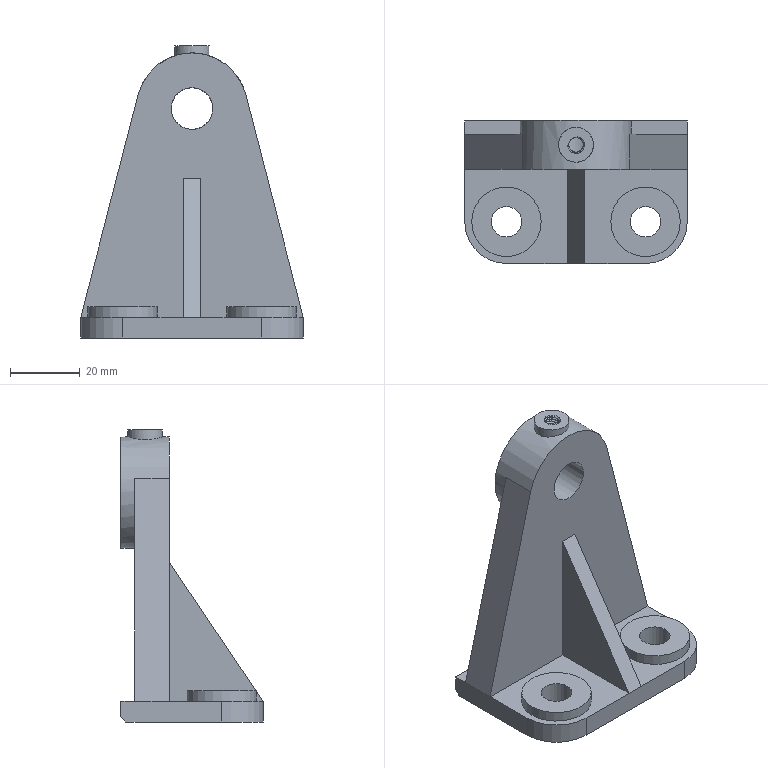Part | NX | features EXTRUDE 7, DATUM_CSYS 6, SKETCH 5, CHAMFER 1, CPROJ 1, CYLINDER 1, Intersection Curve 1, RIB 1, SUBTRACT 1, THREADS 1 | 1 solid | 37 faces | box 64 x 41 x 84 mm | volume 53505 mm3 | plane 20 | cylinder 13 | spline 3 | cone 1 | commonest cylinder face diameters 4.2 x2 5 x2 8.8 x2 20 x2 24 x2 10 x1